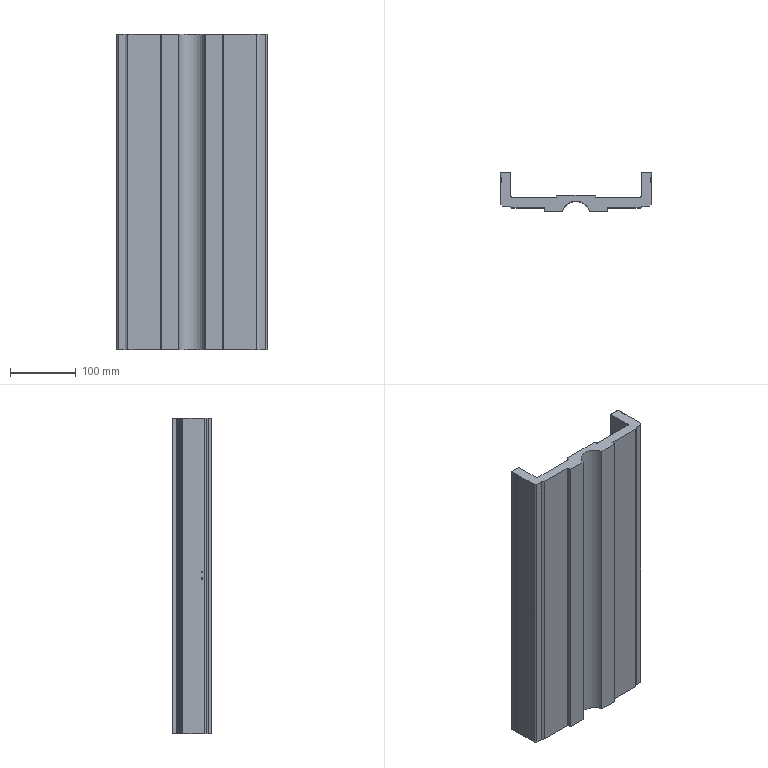Part | SolidWorks | features ICE 9, Fillet 3, HoleWzd 2, Chamfer 1, Cut 1, Extrusion 1, MirrorPattern 1 | 1 solid | 152 faces | box 230 x 60 x 480 mm | volume 2333342 mm3 | cylinder 71 | plane 49 | cone 32 | commonest cylinder face diameters 1 x28 6.8 x24 2.5 x8 2 x4 8 x4 4 x2